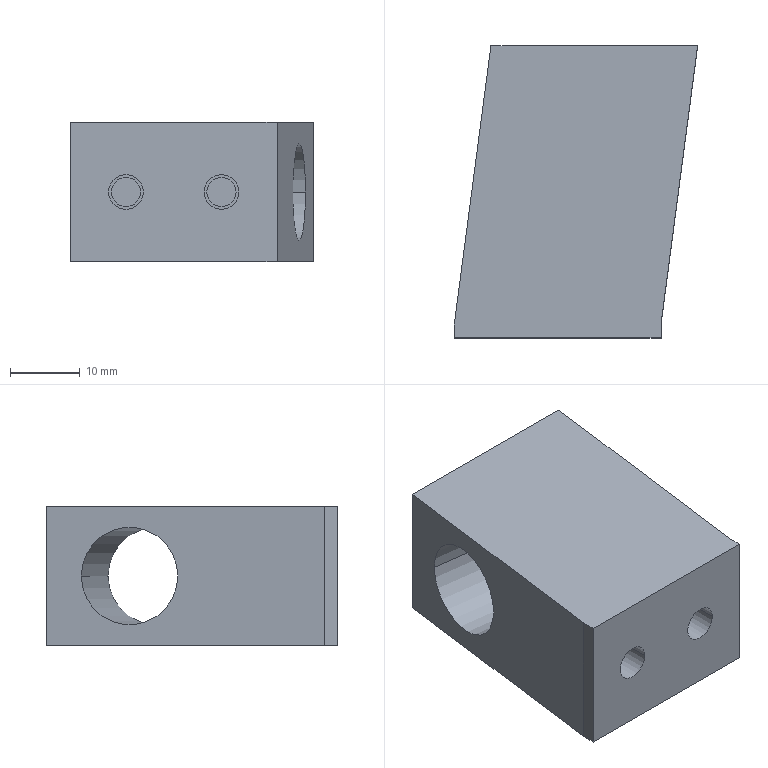Part | SolidWorks | features ICE 4, Extrusion 1 | 1 solid | 22 faces | box 35 x 42 x 20 mm | volume 19935 mm3 | plane 12 | cylinder 10 | commonest cylinder face diameters 4.2 x4 5 x4 14 x2
STEP:
#1=CARTESIAN_POINT('',(-2.058,-9.269,10.));
#2=VERTEX_POINT('',#1);
#3=CARTESIAN_POINT('',(2.142,-9.269,10.));
#4=VERTEX_POINT('',#3);
#5=CARTESIAN_POINT('',(0.04169,-9.269,10.));
#6=DIRECTION('',(0.,-1.,0.));
#7=DIRECTION('',(1.,0.,0.));
#8=AXIS2_PLACEMENT_3D('',#5,#6,#7);
#9=CIRCLE('',#8,2.1);
#10=EDGE_CURVE('',#2,#4,#9,.T.);
#11=ORIENTED_EDGE('',*,*,#10,.F.);
#12=CARTESIAN_POINT('',(-2.058,-13.269,10.));
#13=VERTEX_POINT('',#12);
#14=CARTESIAN_POINT('',(-2.058,-9.269,10.));
#15=DIRECTION('',(0.,-1.,0.));
#16=VECTOR('',#15,1000.);
#17=LINE('',#14,#16);
#18=EDGE_CURVE('',#2,#13,#17,.T.);
#19=ORIENTED_EDGE('',*,*,#18,.T.);
#20=CARTESIAN_POINT('',(2.142,-13.269,10.));
#21=VERTEX_POINT('',#20);
#22=CARTESIAN_POINT('',(0.04169,-13.269,10.));
#23=DIRECTION('',(0.,1.,0.));
#24=DIRECTION('',(1.,0.,0.));
#25=AXIS2_PLACEMENT_3D('',#22,#23,#24);
#26=CIRCLE('',#25,2.1);
#27=EDGE_CURVE('',#21,#13,#26,.T.);
#28=ORIENTED_EDGE('',*,*,#27,.F.);
#29=CARTESIAN_POINT('',(2.142,-9.269,10.));
#30=DIRECTION('',(0.,-1.,0.));
#31=VECTOR('',#30,1000.);
#32=LINE('',#29,#31);
#33=EDGE_CURVE('',#4,#21,#32,.T.);
#34=ORIENTED_EDGE('',*,*,#33,.F.);
#35=EDGE_LOOP('',(#11,#19,#28,#34));
#36=FACE_OUTER_BOUND('',#35,.T.);
#37=CARTESIAN_POINT('',(0.04169,-9.269,10.));
#38=DIRECTION('',(0.,-1.,0.));
#39=DIRECTION('',(1.,0.,0.));
#40=AXIS2_PLACEMENT_3D('',#37,#38,#39);
#41=CYLINDRICAL_SURFACE('',#40,2.1);
#42=ADVANCED_FACE('',(#36),#41,.F.);
#43=CARTESIAN_POINT('',(-15.792,-9.269,10.));
#44=VERTEX_POINT('',#43);
#45=CARTESIAN_POINT('',(-11.592,-9.269,10.));
#46=VERTEX_POINT('',#45);
#47=CARTESIAN_POINT('',(-13.692,-9.269,10.));
#48=DIRECTION('',(0.,-1.,0.));
#49=DIRECTION('',(1.,0.,0.));
#50=AXIS2_PLACEMENT_3D('',#47,#48,#49);
#51=CIRCLE('',#50,2.1);
#52=EDGE_CURVE('',#44,#46,#51,.T.);
#53=ORIENTED_EDGE('',*,*,#52,.F.);
#54=CARTESIAN_POINT('',(-15.792,-13.269,10.));
#55=VERTEX_POINT('',#54);
#56=CARTESIAN_POINT('',(-15.792,-9.269,10.));
#57=DIRECTION('',(0.,-1.,0.));
#58=VECTOR('',#57,1000.);
#59=LINE('',#56,#58);
#60=EDGE_CURVE('',#44,#55,#59,.T.);
#61=ORIENTED_EDGE('',*,*,#60,.T.);
#62=CARTESIAN_POINT('',(-11.592,-13.269,10.));
#63=VERTEX_POINT('',#62);
#64=CARTESIAN_POINT('',(-13.692,-13.269,10.));
#65=DIRECTION('',(0.,1.,0.));
#66=DIRECTION('',(1.,0.,0.));
#67=AXIS2_PLACEMENT_3D('',#64,#65,#66);
#68=CIRCLE('',#67,2.1);
#69=EDGE_CURVE('',#63,#55,#68,.T.);
#70=ORIENTED_EDGE('',*,*,#69,.F.);
#71=CARTESIAN_POINT('',(-11.592,-9.269,10.));
#72=DIRECTION('',(0.,-1.,0.));
#73=VECTOR('',#72,1000.);
#74=LINE('',#71,#73);
#75=EDGE_CURVE('',#46,#63,#74,.T.);
#76=ORIENTED_EDGE('',*,*,#75,.F.);
#77=EDGE_LOOP('',(#53,#61,#70,#76));
#78=FACE_OUTER_BOUND('',#77,.T.);
#79=CARTESIAN_POINT('',(-13.692,-9.269,10.));
#80=DIRECTION('',(0.,-1.,0.));
#81=DIRECTION('',(1.,0.,0.));
#82=AXIS2_PLACEMENT_3D('',#79,#80,#81);
#83=CYLINDRICAL_SURFACE('',#82,2.1);
#84=ADVANCED_FACE('',(#78),#83,.F.);
#85=CARTESIAN_POINT('',(-2.458,-13.269,10.));
#86=VERTEX_POINT('',#85);
#87=CARTESIAN_POINT('',(2.542,-13.269,10.));
#88=VERTEX_POINT('',#87);
#89=CARTESIAN_POINT('',(0.04169,-13.269,10.));
#90=DIRECTION('',(0.,-1.,0.));
#91=DIRECTION('',(1.,0.,0.));
#92=AXIS2_PLACEMENT_3D('',#89,#90,#91);
#93=CIRCLE('',#92,2.5);
#94=EDGE_CURVE('',#86,#88,#93,.T.);
#95=ORIENTED_EDGE('',*,*,#94,.F.);
#96=CARTESIAN_POINT('',(-2.458,-23.269,10.));
#97=VERTEX_POINT('',#96);
#98=CARTESIAN_POINT('',(-2.458,-13.269,10.));
#99=DIRECTION('',(0.,-1.,0.));
#100=VECTOR('',#99,1000.);
#101=LINE('',#98,#100);
#102=EDGE_CURVE('',#86,#97,#101,.T.);
#103=ORIENTED_EDGE('',*,*,#102,.T.);
#104=CARTESIAN_POINT('',(2.542,-23.269,10.));
#105=VERTEX_POINT('',#104);
#106=CARTESIAN_POINT('',(0.04169,-23.269,10.));
#107=DIRECTION('',(0.,-1.,0.));
#108=DIRECTION('',(1.,0.,0.));
#109=AXIS2_PLACEMENT_3D('',#106,#107,#108);
#110=CIRCLE('',#109,2.5);
#111=EDGE_CURVE('',#97,#105,#110,.T.);
#112=ORIENTED_EDGE('',*,*,#111,.T.);
#113=CARTESIAN_POINT('',(2.542,-13.269,10.));
#114=DIRECTION('',(0.,-1.,0.));
#115=VECTOR('',#114,1000.);
#116=LINE('',#113,#115);
#117=EDGE_CURVE('',#88,#105,#116,.T.);
#118=ORIENTED_EDGE('',*,*,#117,.F.);
#119=EDGE_LOOP('',(#95,#103,#112,#118));
#120=FACE_OUTER_BOUND('',#119,.T.);
#121=CARTESIAN_POINT('',(0.04169,-13.269,10.));
#122=DIRECTION('',(0.,-1.,0.));
#123=DIRECTION('',(1.,0.,0.));
#124=AXIS2_PLACEMENT_3D('',#121,#122,#123);
#125=CYLINDRICAL_SURFACE('',#124,2.5);
#126=ADVANCED_FACE('',(#120),#125,.F.);
#127=CARTESIAN_POINT('',(-16.192,-13.269,10.));
#128=VERTEX_POINT('',#127);
#129=CARTESIAN_POINT('',(-11.192,-13.269,10.));
#130=VERTEX_POINT('',#129);
#131=CARTESIAN_POINT('',(-13.692,-13.269,10.));
#132=DIRECTION('',(0.,-1.,0.));
#133=DIRECTION('',(1.,0.,0.));
#134=AXIS2_PLACEMENT_3D('',#131,#132,#133);
#135=CIRCLE('',#134,2.5);
#136=EDGE_CURVE('',#128,#130,#135,.T.);
#137=ORIENTED_EDGE('',*,*,#136,.F.);
#138=CARTESIAN_POINT('',(-16.192,-23.269,10.));
#139=VERTEX_POINT('',#138);
#140=CARTESIAN_POINT('',(-16.192,-13.269,10.));
#141=DIRECTION('',(0.,-1.,0.));
#142=VECTOR('',#141,1000.);
#143=LINE('',#140,#142);
#144=EDGE_CURVE('',#128,#139,#143,.T.);
#145=ORIENTED_EDGE('',*,*,#144,.T.);
#146=CARTESIAN_POINT('',(-11.192,-23.269,10.));
#147=VERTEX_POINT('',#146);
#148=CARTESIAN_POINT('',(-13.692,-23.269,10.));
#149=DIRECTION('',(0.,-1.,0.));
#150=DIRECTION('',(1.,0.,0.));
#151=AXIS2_PLACEMENT_3D('',#148,#149,#150);
#152=CIRCLE('',#151,2.5);
#153=EDGE_CURVE('',#139,#147,#152,.T.);
#154=ORIENTED_EDGE('',*,*,#153,.T.);
#155=CARTESIAN_POINT('',(-11.192,-13.269,10.));
#156=DIRECTION('',(0.,-1.,0.));
#157=VECTOR('',#156,1000.);
#158=LINE('',#155,#157);
#159=EDGE_CURVE('',#130,#147,#158,.T.);
#160=ORIENTED_EDGE('',*,*,#159,.F.);
#161=EDGE_LOOP('',(#137,#145,#154,#160));
#162=FACE_OUTER_BOUND('',#161,.T.);
#163=CARTESIAN_POINT('',(-13.692,-13.269,10.));
#164=DIRECTION('',(0.,-1.,0.));
#165=DIRECTION('',(1.,0.,0.));
#166=AXIS2_PLACEMENT_3D('',#163,#164,#165);
#167=CYLINDRICAL_SURFACE('',#166,2.5);
#168=ADVANCED_FACE('',(#162),#167,.F.);
#169=CARTESIAN_POINT('',(10.306,-4.072,10.));
#170=VERTEX_POINT('',#169);
#171=CARTESIAN_POINT('',(12.133,9.808,10.));
#172=VERTEX_POINT('',#171);
#173=CARTESIAN_POINT('',(11.219,2.868,10.));
#174=DIRECTION('',(0.9914,-0.1305,0.));
#175=DIRECTION('',(-0.1305,-0.9914,0.));
#176=AXIS2_PLACEMENT_3D('',#173,#174,#175);
#177=CIRCLE('',#176,7.);
#178=EDGE_CURVE('',#170,#172,#177,.T.);
#179=ORIENTED_EDGE('',*,*,#178,.T.);
#180=CARTESIAN_POINT('',(-17.094,13.656,10.));
#181=VERTEX_POINT('',#180);
#182=CARTESIAN_POINT('',(17.569,9.092,10.));
#183=DIRECTION('',(-0.9914,0.1305,0.));
#184=VECTOR('',#183,1000.);
#185=LINE('',#182,#184);
#186=EDGE_CURVE('',#172,#181,#185,.T.);
#187=ORIENTED_EDGE('',*,*,#186,.T.);
#188=CARTESIAN_POINT('',(-18.922,-0.2247,10.));
#189=VERTEX_POINT('',#188);
#190=CARTESIAN_POINT('',(-18.008,6.715,10.));
#191=DIRECTION('',(-0.9914,0.1305,0.));
#192=DIRECTION('',(-0.1305,-0.9914,0.));
#193=AXIS2_PLACEMENT_3D('',#190,#191,#192);
#194=CIRCLE('',#193,7.);
#195=EDGE_CURVE('',#181,#189,#194,.T.);
#196=ORIENTED_EDGE('',*,*,#195,.T.);
#197=CARTESIAN_POINT('',(15.742,-4.788,10.));
#198=DIRECTION('',(-0.9914,0.1305,0.));
#199=VECTOR('',#198,1000.);
#200=LINE('',#197,#199);
#201=EDGE_CURVE('',#170,#189,#200,.T.);
#202=ORIENTED_EDGE('',*,*,#201,.F.);
#203=EDGE_LOOP('',(#179,#187,#196,#202));
#204=FACE_OUTER_BOUND('',#203,.T.);
#205=CARTESIAN_POINT('',(16.656,2.152,10.));
#206=DIRECTION('',(-0.9914,0.1305,0.));
#207=DIRECTION('',(-0.1305,-0.9914,0.));
#208=AXIS2_PLACEMENT_3D('',#205,#206,#207);
#209=CYLINDRICAL_SURFACE('',#208,7.);
#210=ADVANCED_FACE('',(#204),#209,.F.);
#211=CARTESIAN_POINT('',(-21.692,-21.269,20.));
#212=VERTEX_POINT('',#211);
#213=CARTESIAN_POINT('',(-21.692,-23.269,20.));
#214=VERTEX_POINT('',#213);
#215=CARTESIAN_POINT('',(-21.692,18.731,20.));
#216=DIRECTION('',(0.,-1.,0.));
#217=VECTOR('',#216,1000.);
#218=LINE('',#215,#217);
#219=EDGE_CURVE('',#212,#214,#218,.T.);
#220=ORIENTED_EDGE('',*,*,#219,.F.);
#221=CARTESIAN_POINT('',(-21.692,-21.269,0.));
#222=VERTEX_POINT('',#221);
#223=CARTESIAN_POINT('',(-21.692,-21.269,-0.001));
#224=DIRECTION('',(0.,0.,1.));
#225=VECTOR('',#224,1000.);
#226=LINE('',#223,#225);
#227=EDGE_CURVE('',#222,#212,#226,.T.);
#228=ORIENTED_EDGE('',*,*,#227,.F.);
#229=CARTESIAN_POINT('',(-21.692,-23.269,0.));
#230=VERTEX_POINT('',#229);
#231=CARTESIAN_POINT('',(-21.692,18.731,0.));
#232=DIRECTION('',(0.,-1.,0.));
#233=VECTOR('',#232,1000.);
#234=LINE('',#231,#233);
#235=EDGE_CURVE('',#222,#230,#234,.T.);
#236=ORIENTED_EDGE('',*,*,#235,.T.);
#237=CARTESIAN_POINT('',(-21.692,-23.269,20.));
#238=DIRECTION('',(0.,0.,-1.));
#239=VECTOR('',#238,1000.);
#240=LINE('',#237,#239);
#241=EDGE_CURVE('',#214,#230,#240,.T.);
#242=ORIENTED_EDGE('',*,*,#241,.F.);
#243=EDGE_LOOP('',(#220,#228,#236,#242));
#244=FACE_OUTER_BOUND('',#243,.T.);
#245=CARTESIAN_POINT('',(-21.692,18.731,20.));
#246=DIRECTION('',(1.,0.,0.));
#247=DIRECTION('',(0.,0.,-1.));
#248=AXIS2_PLACEMENT_3D('',#245,#246,#247);
#249=PLANE('',#248);
#250=ADVANCED_FACE('',(#244),#249,.F.);
#251=CARTESIAN_POINT('',(-13.692,-23.269,10.));
#252=DIRECTION('',(0.,-1.,0.));
#253=DIRECTION('',(1.,0.,0.));
#254=AXIS2_PLACEMENT_3D('',#251,#252,#253);
#255=CIRCLE('',#254,2.5);
#256=EDGE_CURVE('',#147,#139,#255,.T.);
#257=ORIENTED_EDGE('',*,*,#256,.F.);
#258=ORIENTED_EDGE('',*,*,#153,.F.);
#259=EDGE_LOOP('',(#257,#258));
#260=FACE_BOUND('',#259,.T.);
#261=CARTESIAN_POINT('',(0.04169,-23.269,10.));
#262=DIRECTION('',(0.,-1.,0.));
#263=DIRECTION('',(1.,0.,0.));
#264=AXIS2_PLACEMENT_3D('',#261,#262,#263);
#265=CIRCLE('',#264,2.5);
#266=EDGE_CURVE('',#105,#97,#265,.T.);
#267=ORIENTED_EDGE('',*,*,#266,.F.);
#268=ORIENTED_EDGE('',*,*,#111,.F.);
#269=EDGE_LOOP('',(#267,#268));
#270=FACE_BOUND('',#269,.T.);
#271=CARTESIAN_POINT('',(8.042,-23.269,0.));
#272=VERTEX_POINT('',#271);
#273=CARTESIAN_POINT('',(-21.692,-23.269,0.));
#274=DIRECTION('',(1.,0.,0.));
#275=VECTOR('',#274,1000.);
#276=LINE('',#273,#275);
#277=EDGE_CURVE('',#230,#272,#276,.T.);
#278=ORIENTED_EDGE('',*,*,#277,.T.);
#279=CARTESIAN_POINT('',(8.042,-23.269,20.));
#280=VERTEX_POINT('',#279);
#281=CARTESIAN_POINT('',(8.042,-23.269,-0.001));
#282=DIRECTION('',(0.,0.,1.));
#283=VECTOR('',#282,1000.);
#284=LINE('',#281,#283);
#285=EDGE_CURVE('',#272,#280,#284,.T.);
#286=ORIENTED_EDGE('',*,*,#285,.T.);
#287=CARTESIAN_POINT('',(-21.692,-23.269,20.));
#288=DIRECTION('',(1.,0.,0.));
#289=VECTOR('',#288,1000.);
#290=LINE('',#287,#289);
#291=EDGE_CURVE('',#214,#280,#290,.T.);
#292=ORIENTED_EDGE('',*,*,#291,.F.);
#293=ORIENTED_EDGE('',*,*,#241,.T.);
#294=EDGE_LOOP('',(#278,#286,#292,#293));
#295=FACE_OUTER_BOUND('',#294,.T.);
#296=CARTESIAN_POINT('',(-21.692,-23.269,20.));
#297=DIRECTION('',(0.,1.,0.));
#298=DIRECTION('',(-1.,0.,0.));
#299=AXIS2_PLACEMENT_3D('',#296,#297,#298);
#300=PLANE('',#299);
#301=ADVANCED_FACE('',(#260,#270,#295),#300,.F.);
#302=CARTESIAN_POINT('',(13.308,18.731,0.));
#303=VERTEX_POINT('',#302);
#304=CARTESIAN_POINT('',(-16.426,18.731,0.));
#305=VERTEX_POINT('',#304);
#306=CARTESIAN_POINT('',(-21.692,18.731,0.));
#307=DIRECTION('',(-1.,0.,0.));
#308=VECTOR('',#307,1000.);
#309=LINE('',#306,#308);
#310=EDGE_CURVE('',#303,#305,#309,.T.);
#311=ORIENTED_EDGE('',*,*,#310,.T.);
#312=CARTESIAN_POINT('',(-16.426,18.731,20.));
#313=VERTEX_POINT('',#312);
#314=CARTESIAN_POINT('',(-16.426,18.731,-0.001));
#315=DIRECTION('',(0.,0.,1.));
#316=VECTOR('',#315,1000.);
#317=LINE('',#314,#316);
#318=EDGE_CURVE('',#305,#313,#317,.T.);
#319=ORIENTED_EDGE('',*,*,#318,.T.);
#320=CARTESIAN_POINT('',(13.308,18.731,20.));
#321=VERTEX_POINT('',#320);
#322=CARTESIAN_POINT('',(-21.692,18.731,20.));
#323=DIRECTION('',(-1.,0.,0.));
#324=VECTOR('',#323,1000.);
#325=LINE('',#322,#324);
#326=EDGE_CURVE('',#321,#313,#325,.T.);
#327=ORIENTED_EDGE('',*,*,#326,.F.);
#328=CARTESIAN_POINT('',(13.308,18.731,20.));
#329=DIRECTION('',(0.,0.,-1.));
#330=VECTOR('',#329,1000.);
#331=LINE('',#328,#330);
#332=EDGE_CURVE('',#321,#303,#331,.T.);
#333=ORIENTED_EDGE('',*,*,#332,.T.);
#334=EDGE_LOOP('',(#311,#319,#327,#333));
#335=FACE_OUTER_BOUND('',#334,.T.);
#336=CARTESIAN_POINT('',(-21.692,18.731,20.));
#337=DIRECTION('',(0.,-1.,0.));
#338=DIRECTION('',(0.,0.,-1.));
#339=AXIS2_PLACEMENT_3D('',#336,#337,#338);
#340=PLANE('',#339);
#341=ADVANCED_FACE('',(#335),#340,.F.);
#342=CARTESIAN_POINT('',(-16.426,18.731,20.));
#343=DIRECTION('',(0.1305,0.9914,0.));
#344=VECTOR('',#343,1000.);
#345=LINE('',#342,#344);
#346=EDGE_CURVE('',#212,#313,#345,.T.);
#347=ORIENTED_EDGE('',*,*,#346,.F.);
#348=ORIENTED_EDGE('',*,*,#219,.T.);
#349=ORIENTED_EDGE('',*,*,#291,.T.);
#350=CARTESIAN_POINT('',(8.042,-21.269,20.));
#351=VERTEX_POINT('',#350);
#352=CARTESIAN_POINT('',(8.042,-21.269,20.));
#353=DIRECTION('',(0.,-1.,0.));
#354=VECTOR('',#353,1000.);
#355=LINE('',#352,#354);
#356=EDGE_CURVE('',#351,#280,#355,.T.);
#357=ORIENTED_EDGE('',*,*,#356,.F.);
#358=CARTESIAN_POINT('',(13.308,18.731,20.));
#359=DIRECTION('',(-0.1305,-0.9914,0.));
#360=VECTOR('',#359,1000.);
#361=LINE('',#358,#360);
#362=EDGE_CURVE('',#321,#351,#361,.T.);
#363=ORIENTED_EDGE('',*,*,#362,.F.);
#364=ORIENTED_EDGE('',*,*,#326,.T.);
#365=EDGE_LOOP('',(#347,#348,#349,#357,#363,#364));
#366=FACE_OUTER_BOUND('',#365,.T.);
#367=CARTESIAN_POINT('',(0.,0.,20.));
#368=DIRECTION('',(0.,0.,1.));
#369=DIRECTION('',(1.,0.,0.));
#370=AXIS2_PLACEMENT_3D('',#367,#368,#369);
#371=PLANE('',#370);
#372=ADVANCED_FACE('',(#366),#371,.T.);
#373=ORIENTED_EDGE('',*,*,#235,.F.);
#374=CARTESIAN_POINT('',(-16.426,18.731,0.));
#375=DIRECTION('',(-0.1305,-0.9914,0.));
#376=VECTOR('',#375,1000.);
#377=LINE('',#374,#376);
#378=EDGE_CURVE('',#305,#222,#377,.T.);
#379=ORIENTED_EDGE('',*,*,#378,.F.);
#380=ORIENTED_EDGE('',*,*,#310,.F.);
#381=CARTESIAN_POINT('',(8.042,-21.269,0.));
#382=VERTEX_POINT('',#381);
#383=CARTESIAN_POINT('',(13.308,18.731,0.));
#384=DIRECTION('',(0.1305,0.9914,0.));
#385=VECTOR('',#384,1000.);
#386=LINE('',#383,#385);
#387=EDGE_CURVE('',#382,#303,#386,.T.);
#388=ORIENTED_EDGE('',*,*,#387,.F.);
#389=CARTESIAN_POINT('',(8.042,-21.269,0.));
#390=DIRECTION('',(0.,1.,0.));
#391=VECTOR('',#390,1000.);
#392=LINE('',#389,#391);
#393=EDGE_CURVE('',#272,#382,#392,.T.);
#394=ORIENTED_EDGE('',*,*,#393,.F.);
#395=ORIENTED_EDGE('',*,*,#277,.F.);
#396=EDGE_LOOP('',(#373,#379,#380,#388,#394,#395));
#397=FACE_OUTER_BOUND('',#396,.T.);
#398=CARTESIAN_POINT('',(0.,0.,0.));
#399=DIRECTION('',(0.,0.,1.));
#400=DIRECTION('',(1.,0.,0.));
#401=AXIS2_PLACEMENT_3D('',#398,#399,#400);
#402=PLANE('',#401);
#403=ADVANCED_FACE('',(#397),#402,.F.);
#404=ORIENTED_EDGE('',*,*,#393,.T.);
#405=CARTESIAN_POINT('',(8.042,-21.269,-0.001));
#406=DIRECTION('',(0.,0.,1.));
#407=VECTOR('',#406,1000.);
#408=LINE('',#405,#407);
#409=EDGE_CURVE('',#382,#351,#408,.T.);
#410=ORIENTED_EDGE('',*,*,#409,.T.);
#411=ORIENTED_EDGE('',*,*,#356,.T.);
#412=ORIENTED_EDGE('',*,*,#285,.F.);
#413=EDGE_LOOP('',(#404,#410,#411,#412));
#414=FACE_OUTER_BOUND('',#413,.T.);
#415=CARTESIAN_POINT('',(8.042,-21.269,-0.001));
#416=DIRECTION('',(-1.,0.,0.));
#417=DIRECTION('',(0.,0.,1.));
#418=AXIS2_PLACEMENT_3D('',#415,#416,#417);
#419=PLANE('',#418);
#420=ADVANCED_FACE('',(#414),#419,.F.);
#421=ORIENTED_EDGE('',*,*,#178,.F.);
#422=CARTESIAN_POINT('',(11.219,2.868,10.));
#423=DIRECTION('',(0.9914,-0.1305,0.));
#424=DIRECTION('',(-0.1305,-0.9914,0.));
#425=AXIS2_PLACEMENT_3D('',#422,#423,#424);
#426=CIRCLE('',#425,7.);
#427=EDGE_CURVE('',#172,#170,#426,.T.);
#428=ORIENTED_EDGE('',*,*,#427,.F.);
#429=EDGE_LOOP('',(#421,#428));
#430=FACE_BOUND('',#429,.T.);
#431=ORIENTED_EDGE('',*,*,#387,.T.);
#432=ORIENTED_EDGE('',*,*,#332,.F.);
#433=ORIENTED_EDGE('',*,*,#362,.T.);
#434=ORIENTED_EDGE('',*,*,#409,.F.);
#435=EDGE_LOOP('',(#431,#432,#433,#434));
#436=FACE_OUTER_BOUND('',#435,.T.);
#437=CARTESIAN_POINT('',(13.308,18.731,-0.001));
#438=DIRECTION('',(-0.9914,0.1305,0.));
#439=DIRECTION('',(-0.1305,-0.9914,0.));
#440=AXIS2_PLACEMENT_3D('',#437,#438,#439);
#441=PLANE('',#440);
#442=ADVANCED_FACE('',(#430,#436),#441,.F.);
#443=CARTESIAN_POINT('',(-18.008,6.715,10.));
#444=DIRECTION('',(-0.9914,0.1305,0.));
#445=DIRECTION('',(-0.1305,-0.9914,0.));
#446=AXIS2_PLACEMENT_3D('',#443,#444,#445);
#447=CIRCLE('',#446,7.);
#448=EDGE_CURVE('',#189,#181,#447,.T.);
#449=ORIENTED_EDGE('',*,*,#448,.F.);
#450=ORIENTED_EDGE('',*,*,#195,.F.);
#451=EDGE_LOOP('',(#449,#450));
#452=FACE_BOUND('',#451,.T.);
#453=ORIENTED_EDGE('',*,*,#378,.T.);
#454=ORIENTED_EDGE('',*,*,#227,.T.);
#455=ORIENTED_EDGE('',*,*,#346,.T.);
#456=ORIENTED_EDGE('',*,*,#318,.F.);
#457=EDGE_LOOP('',(#453,#454,#455,#456));
#458=FACE_OUTER_BOUND('',#457,.T.);
#459=CARTESIAN_POINT('',(-16.426,18.731,-0.001));
#460=DIRECTION('',(0.9914,-0.1305,0.));
#461=DIRECTION('',(0.1305,0.9914,0.));
#462=AXIS2_PLACEMENT_3D('',#459,#460,#461);
#463=PLANE('',#462);
#464=ADVANCED_FACE('',(#452,#458),#463,.F.);
#465=ORIENTED_EDGE('',*,*,#186,.F.);
#466=ORIENTED_EDGE('',*,*,#427,.T.);
#467=ORIENTED_EDGE('',*,*,#201,.T.);
#468=ORIENTED_EDGE('',*,*,#448,.T.);
#469=EDGE_LOOP('',(#465,#466,#467,#468));
#470=FACE_OUTER_BOUND('',#469,.T.);
#471=CARTESIAN_POINT('',(16.656,2.152,10.));
#472=DIRECTION('',(-0.9914,0.1305,0.));
#473=DIRECTION('',(-0.1305,-0.9914,0.));
#474=AXIS2_PLACEMENT_3D('',#471,#472,#473);
#475=CYLINDRICAL_SURFACE('',#474,7.);
#476=ADVANCED_FACE('',(#470),#475,.F.);
#477=CARTESIAN_POINT('',(-13.692,-13.269,10.));
#478=DIRECTION('',(0.,-1.,0.));
#479=DIRECTION('',(1.,0.,0.));
#480=AXIS2_PLACEMENT_3D('',#477,#478,#479);
#481=CIRCLE('',#480,2.5);
#482=EDGE_CURVE('',#130,#128,#481,.T.);
#483=ORIENTED_EDGE('',*,*,#482,.T.);
#484=ORIENTED_EDGE('',*,*,#136,.T.);
#485=EDGE_LOOP('',(#483,#484));
#486=FACE_OUTER_BOUND('',#485,.T.);
#487=ORIENTED_EDGE('',*,*,#69,.T.);
#488=CARTESIAN_POINT('',(-13.692,-13.269,10.));
#489=DIRECTION('',(0.,1.,0.));
#490=DIRECTION('',(1.,0.,0.));
#491=AXIS2_PLACEMENT_3D('',#488,#489,#490);
#492=CIRCLE('',#491,2.1);
#493=EDGE_CURVE('',#55,#63,#492,.T.);
#494=ORIENTED_EDGE('',*,*,#493,.T.);
#495=EDGE_LOOP('',(#487,#494));
#496=FACE_BOUND('',#495,.T.);
#497=CARTESIAN_POINT('',(-13.692,-13.269,10.));
#498=DIRECTION('',(0.,-1.,0.));
#499=DIRECTION('',(1.,0.,0.));
#500=AXIS2_PLACEMENT_3D('',#497,#498,#499);
#501=PLANE('',#500);
#502=ADVANCED_FACE('',(#486,#496),#501,.T.);
#503=ORIENTED_EDGE('',*,*,#144,.F.);
#504=ORIENTED_EDGE('',*,*,#482,.F.);
#505=ORIENTED_EDGE('',*,*,#159,.T.);
#506=ORIENTED_EDGE('',*,*,#256,.T.);
#507=EDGE_LOOP('',(#503,#504,#505,#506));
#508=FACE_OUTER_BOUND('',#507,.T.);
#509=CARTESIAN_POINT('',(-13.692,-13.269,10.));
#510=DIRECTION('',(0.,-1.,0.));
#511=DIRECTION('',(1.,0.,0.));
#512=AXIS2_PLACEMENT_3D('',#509,#510,#511);
#513=CYLINDRICAL_SURFACE('',#512,2.5);
#514=ADVANCED_FACE('',(#508),#513,.F.);
#515=CARTESIAN_POINT('',(0.04169,-13.269,10.));
#516=DIRECTION('',(0.,-1.,0.));
#517=DIRECTION('',(1.,0.,0.));
#518=AXIS2_PLACEMENT_3D('',#515,#516,#517);
#519=CIRCLE('',#518,2.5);
#520=EDGE_CURVE('',#88,#86,#519,.T.);
#521=ORIENTED_EDGE('',*,*,#520,.T.);
#522=ORIENTED_EDGE('',*,*,#94,.T.);
#523=EDGE_LOOP('',(#521,#522));
#524=FACE_OUTER_BOUND('',#523,.T.);
#525=ORIENTED_EDGE('',*,*,#27,.T.);
#526=CARTESIAN_POINT('',(0.04169,-13.269,10.));
#527=DIRECTION('',(0.,1.,0.));
#528=DIRECTION('',(1.,0.,0.));
#529=AXIS2_PLACEMENT_3D('',#526,#527,#528);
#530=CIRCLE('',#529,2.1);
#531=EDGE_CURVE('',#13,#21,#530,.T.);
#532=ORIENTED_EDGE('',*,*,#531,.T.);
#533=EDGE_LOOP('',(#525,#532));
#534=FACE_BOUND('',#533,.T.);
#535=CARTESIAN_POINT('',(0.04169,-13.269,10.));
#536=DIRECTION('',(0.,-1.,0.));
#537=DIRECTION('',(1.,0.,0.));
#538=AXIS2_PLACEMENT_3D('',#535,#536,#537);
#539=PLANE('',#538);
#540=ADVANCED_FACE('',(#524,#534),#539,.T.);
#541=ORIENTED_EDGE('',*,*,#102,.F.);
#542=ORIENTED_EDGE('',*,*,#520,.F.);
#543=ORIENTED_EDGE('',*,*,#117,.T.);
#544=ORIENTED_EDGE('',*,*,#266,.T.);
#545=EDGE_LOOP('',(#541,#542,#543,#544));
#546=FACE_OUTER_BOUND('',#545,.T.);
#547=CARTESIAN_POINT('',(0.04169,-13.269,10.));
#548=DIRECTION('',(0.,-1.,0.));
#549=DIRECTION('',(1.,0.,0.));
#550=AXIS2_PLACEMENT_3D('',#547,#548,#549);
#551=CYLINDRICAL_SURFACE('',#550,2.5);
#552=ADVANCED_FACE('',(#546),#551,.F.);
#553=CARTESIAN_POINT('',(-13.692,-9.269,10.));
#554=DIRECTION('',(0.,-1.,0.));
#555=DIRECTION('',(1.,0.,0.));
#556=AXIS2_PLACEMENT_3D('',#553,#554,#555);
#557=CIRCLE('',#556,2.1);
#558=EDGE_CURVE('',#46,#44,#557,.T.);
#559=ORIENTED_EDGE('',*,*,#558,.T.);
#560=ORIENTED_EDGE('',*,*,#52,.T.);
#561=EDGE_LOOP('',(#559,#560));
#562=FACE_OUTER_BOUND('',#561,.T.);
#563=CARTESIAN_POINT('',(-13.692,-9.269,10.));
#564=DIRECTION('',(0.,-1.,0.));
#565=DIRECTION('',(1.,0.,0.));
#566=AXIS2_PLACEMENT_3D('',#563,#564,#565);
#567=PLANE('',#566);
#568=ADVANCED_FACE('',(#562),#567,.T.);
#569=ORIENTED_EDGE('',*,*,#60,.F.);
#570=ORIENTED_EDGE('',*,*,#558,.F.);
#571=ORIENTED_EDGE('',*,*,#75,.T.);
#572=ORIENTED_EDGE('',*,*,#493,.F.);
#573=EDGE_LOOP('',(#569,#570,#571,#572));
#574=FACE_OUTER_BOUND('',#573,.T.);
#575=CARTESIAN_POINT('',(-13.692,-9.269,10.));
#576=DIRECTION('',(0.,-1.,0.));
#577=DIRECTION('',(1.,0.,0.));
#578=AXIS2_PLACEMENT_3D('',#575,#576,#577);
#579=CYLINDRICAL_SURFACE('',#578,2.1);
#580=ADVANCED_FACE('',(#574),#579,.F.);
#581=CARTESIAN_POINT('',(0.04169,-9.269,10.));
#582=DIRECTION('',(0.,-1.,0.));
#583=DIRECTION('',(1.,0.,0.));
#584=AXIS2_PLACEMENT_3D('',#581,#582,#583);
#585=CIRCLE('',#584,2.1);
#586=EDGE_CURVE('',#4,#2,#585,.T.);
#587=ORIENTED_EDGE('',*,*,#586,.T.);
#588=ORIENTED_EDGE('',*,*,#10,.T.);
#589=EDGE_LOOP('',(#587,#588));
#590=FACE_OUTER_BOUND('',#589,.T.);
#591=CARTESIAN_POINT('',(0.04169,-9.269,10.));
#592=DIRECTION('',(0.,-1.,0.));
#593=DIRECTION('',(1.,0.,0.));
#594=AXIS2_PLACEMENT_3D('',#591,#592,#593);
#595=PLANE('',#594);
#596=ADVANCED_FACE('',(#590),#595,.T.);
#597=ORIENTED_EDGE('',*,*,#18,.F.);
#598=ORIENTED_EDGE('',*,*,#586,.F.);
#599=ORIENTED_EDGE('',*,*,#33,.T.);
#600=ORIENTED_EDGE('',*,*,#531,.F.);
#601=EDGE_LOOP('',(#597,#598,#599,#600));
#602=FACE_OUTER_BOUND('',#601,.T.);
#603=CARTESIAN_POINT('',(0.04169,-9.269,10.));
#604=DIRECTION('',(0.,-1.,0.));
#605=DIRECTION('',(1.,0.,0.));
#606=AXIS2_PLACEMENT_3D('',#603,#604,#605);
#607=CYLINDRICAL_SURFACE('',#606,2.1);
#608=ADVANCED_FACE('',(#602),#607,.F.);
#609=CLOSED_SHELL('',(#42,#84,#126,#168,#210,#250,#301,#341,#372,#403,#420,#442,#464,#476,#502,#514,#540,#552,#568,#580,#596,#608));
#610=MANIFOLD_SOLID_BREP('',#609);
#611=CARTESIAN_POINT('',(0.,0.,0.));
#612=DIRECTION('',(0.,0.,1.));
#613=DIRECTION('',(1.,0.,0.));
#614=AXIS2_PLACEMENT_3D('',#611,#612,#613);
#615=(LENGTH_UNIT()NAMED_UNIT(*)SI_UNIT(.MILLI.,.METRE.));
#616=UNCERTAINTY_MEASURE_WITH_UNIT(LENGTH_MEASURE(0.00001),#615,'','');
#617=(NAMED_UNIT(*)PLANE_ANGLE_UNIT()SI_UNIT($,.RADIAN.));
#618=(NAMED_UNIT(*)SI_UNIT($,.STERADIAN.)SOLID_ANGLE_UNIT());
#619=(GEOMETRIC_REPRESENTATION_CONTEXT(3)GLOBAL_UNCERTAINTY_ASSIGNED_CONTEXT((#616))GLOBAL_UNIT_ASSIGNED_CONTEXT((#615,#617,#618))REPRESENTATION_CONTEXT('',''));
#620=ADVANCED_BREP_SHAPE_REPRESENTATION('',(#610,#614),#619);